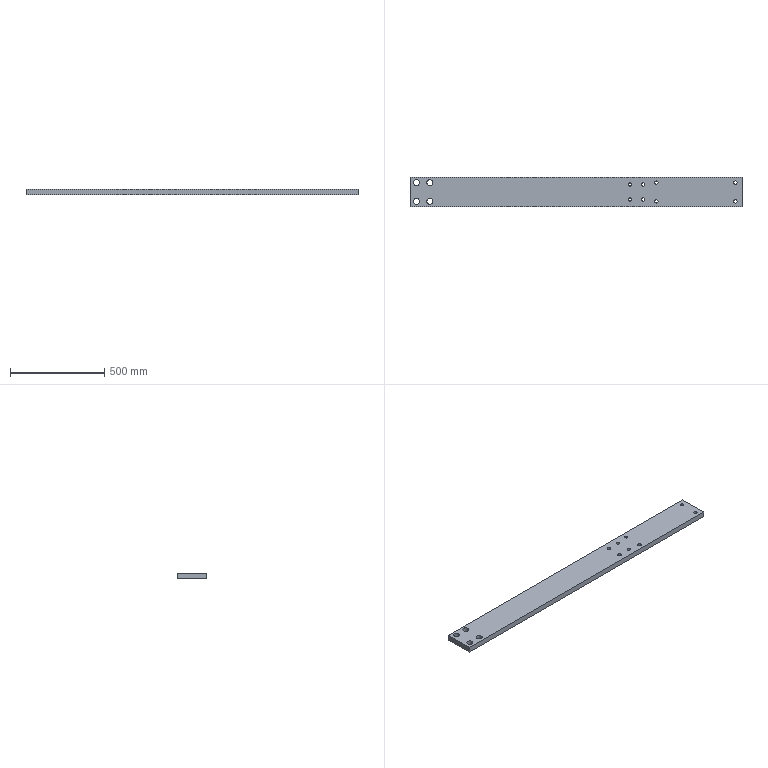Part | NX | features BREP 1 | 1 solid | 30 faces | box 1764 x 158 x 30 mm | volume 8203778 mm3 | cylinder 24 | plane 6 | commonest cylinder face diameters 18 x16 32 x8
STEP:
#1=CARTESIAN_POINT('',(-1230.5,-50.,-15.));
#2=VERTEX_POINT('',#1);
#3=CARTESIAN_POINT('',(-1198.5,-50.,-15.));
#4=VERTEX_POINT('',#3);
#5=CARTESIAN_POINT('',(-1214.5,-50.,-15.));
#6=DIRECTION('',(0.,0.,1.));
#7=DIRECTION('',(-1.,0.,0.));
#8=AXIS2_PLACEMENT_3D('',#5,#6,#7);
#9=CIRCLE('',#8,16.);
#10=EDGE_CURVE('',#2,#4,#9,.T.);
#11=ORIENTED_EDGE('',*,*,#10,.F.);
#12=CARTESIAN_POINT('',(-1230.5,-50.,15.));
#13=VERTEX_POINT('',#12);
#14=CARTESIAN_POINT('',(-1230.5,-50.,-15.));
#15=DIRECTION('',(0.,0.,1.));
#16=VECTOR('',#15,1000.);
#17=LINE('',#14,#16);
#18=EDGE_CURVE('',#2,#13,#17,.T.);
#19=ORIENTED_EDGE('',*,*,#18,.T.);
#20=CARTESIAN_POINT('',(-1198.5,-50.,15.));
#21=VERTEX_POINT('',#20);
#22=CARTESIAN_POINT('',(-1214.5,-50.,15.));
#23=DIRECTION('',(0.,0.,1.));
#24=DIRECTION('',(-1.,0.,0.));
#25=AXIS2_PLACEMENT_3D('',#22,#23,#24);
#26=CIRCLE('',#25,16.);
#27=EDGE_CURVE('',#13,#21,#26,.T.);
#28=ORIENTED_EDGE('',*,*,#27,.T.);
#29=CARTESIAN_POINT('',(-1198.5,-50.,-15.));
#30=DIRECTION('',(0.,0.,1.));
#31=VECTOR('',#30,1000.);
#32=LINE('',#29,#31);
#33=EDGE_CURVE('',#4,#21,#32,.T.);
#34=ORIENTED_EDGE('',*,*,#33,.F.);
#35=EDGE_LOOP('',(#11,#19,#28,#34));
#36=FACE_BOUND('',#35,.T.);
#37=CARTESIAN_POINT('',(-1214.5,-50.,-15.));
#38=DIRECTION('',(0.,0.,1.));
#39=DIRECTION('',(-1.,0.,0.));
#40=AXIS2_PLACEMENT_3D('',#37,#38,#39);
#41=CYLINDRICAL_SURFACE('',#40,16.);
#42=ADVANCED_FACE('',(#36),#41,.F.);
#43=CARTESIAN_POINT('',(-1160.5,-50.,-15.));
#44=VERTEX_POINT('',#43);
#45=CARTESIAN_POINT('',(-1128.5,-50.,-15.));
#46=VERTEX_POINT('',#45);
#47=CARTESIAN_POINT('',(-1144.5,-50.,-15.));
#48=DIRECTION('',(0.,0.,1.));
#49=DIRECTION('',(-1.,0.,0.));
#50=AXIS2_PLACEMENT_3D('',#47,#48,#49);
#51=CIRCLE('',#50,16.);
#52=EDGE_CURVE('',#44,#46,#51,.T.);
#53=ORIENTED_EDGE('',*,*,#52,.F.);
#54=CARTESIAN_POINT('',(-1160.5,-50.,15.));
#55=VERTEX_POINT('',#54);
#56=CARTESIAN_POINT('',(-1160.5,-50.,-15.));
#57=DIRECTION('',(0.,0.,1.));
#58=VECTOR('',#57,1000.);
#59=LINE('',#56,#58);
#60=EDGE_CURVE('',#44,#55,#59,.T.);
#61=ORIENTED_EDGE('',*,*,#60,.T.);
#62=CARTESIAN_POINT('',(-1128.5,-50.,15.));
#63=VERTEX_POINT('',#62);
#64=CARTESIAN_POINT('',(-1144.5,-50.,15.));
#65=DIRECTION('',(0.,0.,1.));
#66=DIRECTION('',(-1.,0.,0.));
#67=AXIS2_PLACEMENT_3D('',#64,#65,#66);
#68=CIRCLE('',#67,16.);
#69=EDGE_CURVE('',#55,#63,#68,.T.);
#70=ORIENTED_EDGE('',*,*,#69,.T.);
#71=CARTESIAN_POINT('',(-1128.5,-50.,-15.));
#72=DIRECTION('',(0.,0.,1.));
#73=VECTOR('',#72,1000.);
#74=LINE('',#71,#73);
#75=EDGE_CURVE('',#46,#63,#74,.T.);
#76=ORIENTED_EDGE('',*,*,#75,.F.);
#77=EDGE_LOOP('',(#53,#61,#70,#76));
#78=FACE_BOUND('',#77,.T.);
#79=CARTESIAN_POINT('',(-1144.5,-50.,-15.));
#80=DIRECTION('',(0.,0.,1.));
#81=DIRECTION('',(-1.,0.,0.));
#82=AXIS2_PLACEMENT_3D('',#79,#80,#81);
#83=CYLINDRICAL_SURFACE('',#82,16.);
#84=ADVANCED_FACE('',(#78),#83,.F.);
#85=CARTESIAN_POINT('',(-1160.5,50.,-15.));
#86=VERTEX_POINT('',#85);
#87=CARTESIAN_POINT('',(-1128.5,50.,-15.));
#88=VERTEX_POINT('',#87);
#89=CARTESIAN_POINT('',(-1144.5,50.,-15.));
#90=DIRECTION('',(0.,0.,1.));
#91=DIRECTION('',(1.,0.,0.));
#92=AXIS2_PLACEMENT_3D('',#89,#90,#91);
#93=CIRCLE('',#92,16.);
#94=EDGE_CURVE('',#86,#88,#93,.T.);
#95=ORIENTED_EDGE('',*,*,#94,.F.);
#96=CARTESIAN_POINT('',(-1160.5,50.,15.));
#97=VERTEX_POINT('',#96);
#98=CARTESIAN_POINT('',(-1160.5,50.,-15.));
#99=DIRECTION('',(0.,0.,1.));
#100=VECTOR('',#99,1000.);
#101=LINE('',#98,#100);
#102=EDGE_CURVE('',#86,#97,#101,.T.);
#103=ORIENTED_EDGE('',*,*,#102,.T.);
#104=CARTESIAN_POINT('',(-1128.5,50.,15.));
#105=VERTEX_POINT('',#104);
#106=CARTESIAN_POINT('',(-1144.5,50.,15.));
#107=DIRECTION('',(0.,0.,1.));
#108=DIRECTION('',(1.,0.,0.));
#109=AXIS2_PLACEMENT_3D('',#106,#107,#108);
#110=CIRCLE('',#109,16.);
#111=EDGE_CURVE('',#97,#105,#110,.T.);
#112=ORIENTED_EDGE('',*,*,#111,.T.);
#113=CARTESIAN_POINT('',(-1128.5,50.,-15.));
#114=DIRECTION('',(0.,0.,1.));
#115=VECTOR('',#114,1000.);
#116=LINE('',#113,#115);
#117=EDGE_CURVE('',#88,#105,#116,.T.);
#118=ORIENTED_EDGE('',*,*,#117,.F.);
#119=EDGE_LOOP('',(#95,#103,#112,#118));
#120=FACE_BOUND('',#119,.T.);
#121=CARTESIAN_POINT('',(-1144.5,50.,-15.));
#122=DIRECTION('',(0.,0.,1.));
#123=DIRECTION('',(-1.,0.,0.));
#124=AXIS2_PLACEMENT_3D('',#121,#122,#123);
#125=CYLINDRICAL_SURFACE('',#124,16.);
#126=ADVANCED_FACE('',(#120),#125,.F.);
#127=CARTESIAN_POINT('',(-1230.5,50.,-15.));
#128=VERTEX_POINT('',#127);
#129=CARTESIAN_POINT('',(-1198.5,50.,-15.));
#130=VERTEX_POINT('',#129);
#131=CARTESIAN_POINT('',(-1214.5,50.,-15.));
#132=DIRECTION('',(0.,0.,1.));
#133=DIRECTION('',(1.,0.,0.));
#134=AXIS2_PLACEMENT_3D('',#131,#132,#133);
#135=CIRCLE('',#134,16.);
#136=EDGE_CURVE('',#128,#130,#135,.T.);
#137=ORIENTED_EDGE('',*,*,#136,.F.);
#138=CARTESIAN_POINT('',(-1230.5,50.,15.));
#139=VERTEX_POINT('',#138);
#140=CARTESIAN_POINT('',(-1230.5,50.,-15.));
#141=DIRECTION('',(0.,0.,1.));
#142=VECTOR('',#141,1000.);
#143=LINE('',#140,#142);
#144=EDGE_CURVE('',#128,#139,#143,.T.);
#145=ORIENTED_EDGE('',*,*,#144,.T.);
#146=CARTESIAN_POINT('',(-1198.5,50.,15.));
#147=VERTEX_POINT('',#146);
#148=CARTESIAN_POINT('',(-1214.5,50.,15.));
#149=DIRECTION('',(0.,0.,1.));
#150=DIRECTION('',(1.,0.,0.));
#151=AXIS2_PLACEMENT_3D('',#148,#149,#150);
#152=CIRCLE('',#151,16.);
#153=EDGE_CURVE('',#139,#147,#152,.T.);
#154=ORIENTED_EDGE('',*,*,#153,.T.);
#155=CARTESIAN_POINT('',(-1198.5,50.,-15.));
#156=DIRECTION('',(0.,0.,1.));
#157=VECTOR('',#156,1000.);
#158=LINE('',#155,#157);
#159=EDGE_CURVE('',#130,#147,#158,.T.);
#160=ORIENTED_EDGE('',*,*,#159,.F.);
#161=EDGE_LOOP('',(#137,#145,#154,#160));
#162=FACE_BOUND('',#161,.T.);
#163=CARTESIAN_POINT('',(-1214.5,50.,-15.));
#164=DIRECTION('',(0.,0.,1.));
#165=DIRECTION('',(-1.,0.,0.));
#166=AXIS2_PLACEMENT_3D('',#163,#164,#165);
#167=CYLINDRICAL_SURFACE('',#166,16.);
#168=ADVANCED_FACE('',(#162),#167,.F.);
#169=CARTESIAN_POINT('',(-89.5,-40.,-15.));
#170=VERTEX_POINT('',#169);
#171=CARTESIAN_POINT('',(-71.5,-40.,-15.));
#172=VERTEX_POINT('',#171);
#173=CARTESIAN_POINT('',(-80.5,-40.,-15.));
#174=DIRECTION('',(0.,0.,1.));
#175=DIRECTION('',(1.,0.,0.));
#176=AXIS2_PLACEMENT_3D('',#173,#174,#175);
#177=CIRCLE('',#176,9.);
#178=EDGE_CURVE('',#170,#172,#177,.T.);
#179=ORIENTED_EDGE('',*,*,#178,.F.);
#180=CARTESIAN_POINT('',(-89.5,-40.,15.));
#181=VERTEX_POINT('',#180);
#182=CARTESIAN_POINT('',(-89.5,-40.,-15.));
#183=DIRECTION('',(0.,0.,1.));
#184=VECTOR('',#183,1000.);
#185=LINE('',#182,#184);
#186=EDGE_CURVE('',#170,#181,#185,.T.);
#187=ORIENTED_EDGE('',*,*,#186,.T.);
#188=CARTESIAN_POINT('',(-71.5,-40.,15.));
#189=VERTEX_POINT('',#188);
#190=CARTESIAN_POINT('',(-80.5,-40.,15.));
#191=DIRECTION('',(0.,0.,1.));
#192=DIRECTION('',(1.,0.,0.));
#193=AXIS2_PLACEMENT_3D('',#190,#191,#192);
#194=CIRCLE('',#193,9.);
#195=EDGE_CURVE('',#181,#189,#194,.T.);
#196=ORIENTED_EDGE('',*,*,#195,.T.);
#197=CARTESIAN_POINT('',(-71.5,-40.,-15.));
#198=DIRECTION('',(0.,0.,1.));
#199=VECTOR('',#198,1000.);
#200=LINE('',#197,#199);
#201=EDGE_CURVE('',#172,#189,#200,.T.);
#202=ORIENTED_EDGE('',*,*,#201,.F.);
#203=EDGE_LOOP('',(#179,#187,#196,#202));
#204=FACE_BOUND('',#203,.T.);
#205=CARTESIAN_POINT('',(-80.5,-40.,-15.));
#206=DIRECTION('',(0.,0.,1.));
#207=DIRECTION('',(-1.,0.,0.));
#208=AXIS2_PLACEMENT_3D('',#205,#206,#207);
#209=CYLINDRICAL_SURFACE('',#208,9.);
#210=ADVANCED_FACE('',(#204),#209,.F.);
#211=CARTESIAN_POINT('',(-19.5,-40.,-15.));
#212=VERTEX_POINT('',#211);
#213=CARTESIAN_POINT('',(-1.5,-40.,-15.));
#214=VERTEX_POINT('',#213);
#215=CARTESIAN_POINT('',(-10.5,-40.,-15.));
#216=DIRECTION('',(0.,0.,1.));
#217=DIRECTION('',(1.,0.,0.));
#218=AXIS2_PLACEMENT_3D('',#215,#216,#217);
#219=CIRCLE('',#218,9.);
#220=EDGE_CURVE('',#212,#214,#219,.T.);
#221=ORIENTED_EDGE('',*,*,#220,.F.);
#222=CARTESIAN_POINT('',(-19.5,-40.,15.));
#223=VERTEX_POINT('',#222);
#224=CARTESIAN_POINT('',(-19.5,-40.,-15.));
#225=DIRECTION('',(0.,0.,1.));
#226=VECTOR('',#225,1000.);
#227=LINE('',#224,#226);
#228=EDGE_CURVE('',#212,#223,#227,.T.);
#229=ORIENTED_EDGE('',*,*,#228,.T.);
#230=CARTESIAN_POINT('',(-1.5,-40.,15.));
#231=VERTEX_POINT('',#230);
#232=CARTESIAN_POINT('',(-10.5,-40.,15.));
#233=DIRECTION('',(0.,0.,1.));
#234=DIRECTION('',(1.,0.,0.));
#235=AXIS2_PLACEMENT_3D('',#232,#233,#234);
#236=CIRCLE('',#235,9.);
#237=EDGE_CURVE('',#223,#231,#236,.T.);
#238=ORIENTED_EDGE('',*,*,#237,.T.);
#239=CARTESIAN_POINT('',(-1.5,-40.,-15.));
#240=DIRECTION('',(0.,0.,1.));
#241=VECTOR('',#240,1000.);
#242=LINE('',#239,#241);
#243=EDGE_CURVE('',#214,#231,#242,.T.);
#244=ORIENTED_EDGE('',*,*,#243,.F.);
#245=EDGE_LOOP('',(#221,#229,#238,#244));
#246=FACE_BOUND('',#245,.T.);
#247=CARTESIAN_POINT('',(-10.5,-40.,-15.));
#248=DIRECTION('',(0.,0.,1.));
#249=DIRECTION('',(-1.,0.,0.));
#250=AXIS2_PLACEMENT_3D('',#247,#248,#249);
#251=CYLINDRICAL_SURFACE('',#250,9.);
#252=ADVANCED_FACE('',(#246),#251,.F.);
#253=CARTESIAN_POINT('',(-89.5,40.,-15.));
#254=VERTEX_POINT('',#253);
#255=CARTESIAN_POINT('',(-71.5,40.,-15.));
#256=VERTEX_POINT('',#255);
#257=CARTESIAN_POINT('',(-80.5,40.,-15.));
#258=DIRECTION('',(0.,0.,1.));
#259=DIRECTION('',(1.,0.,0.));
#260=AXIS2_PLACEMENT_3D('',#257,#258,#259);
#261=CIRCLE('',#260,9.);
#262=EDGE_CURVE('',#254,#256,#261,.T.);
#263=ORIENTED_EDGE('',*,*,#262,.F.);
#264=CARTESIAN_POINT('',(-89.5,40.,15.));
#265=VERTEX_POINT('',#264);
#266=CARTESIAN_POINT('',(-89.5,40.,-15.));
#267=DIRECTION('',(0.,0.,1.));
#268=VECTOR('',#267,1000.);
#269=LINE('',#266,#268);
#270=EDGE_CURVE('',#254,#265,#269,.T.);
#271=ORIENTED_EDGE('',*,*,#270,.T.);
#272=CARTESIAN_POINT('',(-71.5,40.,15.));
#273=VERTEX_POINT('',#272);
#274=CARTESIAN_POINT('',(-80.5,40.,15.));
#275=DIRECTION('',(0.,0.,1.));
#276=DIRECTION('',(1.,0.,0.));
#277=AXIS2_PLACEMENT_3D('',#274,#275,#276);
#278=CIRCLE('',#277,9.);
#279=EDGE_CURVE('',#265,#273,#278,.T.);
#280=ORIENTED_EDGE('',*,*,#279,.T.);
#281=CARTESIAN_POINT('',(-71.5,40.,-15.));
#282=DIRECTION('',(0.,0.,1.));
#283=VECTOR('',#282,1000.);
#284=LINE('',#281,#283);
#285=EDGE_CURVE('',#256,#273,#284,.T.);
#286=ORIENTED_EDGE('',*,*,#285,.F.);
#287=EDGE_LOOP('',(#263,#271,#280,#286));
#288=FACE_BOUND('',#287,.T.);
#289=CARTESIAN_POINT('',(-80.5,40.,-15.));
#290=DIRECTION('',(0.,0.,1.));
#291=DIRECTION('',(-1.,0.,0.));
#292=AXIS2_PLACEMENT_3D('',#289,#290,#291);
#293=CYLINDRICAL_SURFACE('',#292,9.);
#294=ADVANCED_FACE('',(#288),#293,.F.);
#295=CARTESIAN_POINT('',(-19.5,40.,-15.));
#296=VERTEX_POINT('',#295);
#297=CARTESIAN_POINT('',(-1.5,40.,-15.));
#298=VERTEX_POINT('',#297);
#299=CARTESIAN_POINT('',(-10.5,40.,-15.));
#300=DIRECTION('',(0.,0.,1.));
#301=DIRECTION('',(1.,0.,0.));
#302=AXIS2_PLACEMENT_3D('',#299,#300,#301);
#303=CIRCLE('',#302,9.);
#304=EDGE_CURVE('',#296,#298,#303,.T.);
#305=ORIENTED_EDGE('',*,*,#304,.F.);
#306=CARTESIAN_POINT('',(-19.5,40.,15.));
#307=VERTEX_POINT('',#306);
#308=CARTESIAN_POINT('',(-19.5,40.,-15.));
#309=DIRECTION('',(0.,0.,1.));
#310=VECTOR('',#309,1000.);
#311=LINE('',#308,#310);
#312=EDGE_CURVE('',#296,#307,#311,.T.);
#313=ORIENTED_EDGE('',*,*,#312,.T.);
#314=CARTESIAN_POINT('',(-1.5,40.,15.));
#315=VERTEX_POINT('',#314);
#316=CARTESIAN_POINT('',(-10.5,40.,15.));
#317=DIRECTION('',(0.,0.,1.));
#318=DIRECTION('',(1.,0.,0.));
#319=AXIS2_PLACEMENT_3D('',#316,#317,#318);
#320=CIRCLE('',#319,9.);
#321=EDGE_CURVE('',#307,#315,#320,.T.);
#322=ORIENTED_EDGE('',*,*,#321,.T.);
#323=CARTESIAN_POINT('',(-1.5,40.,-15.));
#324=DIRECTION('',(0.,0.,1.));
#325=VECTOR('',#324,1000.);
#326=LINE('',#323,#325);
#327=EDGE_CURVE('',#298,#315,#326,.T.);
#328=ORIENTED_EDGE('',*,*,#327,.F.);
#329=EDGE_LOOP('',(#305,#313,#322,#328));
#330=FACE_BOUND('',#329,.T.);
#331=CARTESIAN_POINT('',(-10.5,40.,-15.));
#332=DIRECTION('',(0.,0.,1.));
#333=DIRECTION('',(-1.,0.,0.));
#334=AXIS2_PLACEMENT_3D('',#331,#332,#333);
#335=CYLINDRICAL_SURFACE('',#334,9.);
#336=ADVANCED_FACE('',(#330),#335,.F.);
#337=CARTESIAN_POINT('',(50.5,-50.,-15.));
#338=VERTEX_POINT('',#337);
#339=CARTESIAN_POINT('',(68.5,-50.,-15.));
#340=VERTEX_POINT('',#339);
#341=CARTESIAN_POINT('',(59.5,-50.,-15.));
#342=DIRECTION('',(0.,0.,1.));
#343=DIRECTION('',(1.,0.,0.));
#344=AXIS2_PLACEMENT_3D('',#341,#342,#343);
#345=CIRCLE('',#344,9.);
#346=EDGE_CURVE('',#338,#340,#345,.T.);
#347=ORIENTED_EDGE('',*,*,#346,.F.);
#348=CARTESIAN_POINT('',(50.5,-50.,15.));
#349=VERTEX_POINT('',#348);
#350=CARTESIAN_POINT('',(50.5,-50.,-15.));
#351=DIRECTION('',(0.,0.,1.));
#352=VECTOR('',#351,1000.);
#353=LINE('',#350,#352);
#354=EDGE_CURVE('',#338,#349,#353,.T.);
#355=ORIENTED_EDGE('',*,*,#354,.T.);
#356=CARTESIAN_POINT('',(68.5,-50.,15.));
#357=VERTEX_POINT('',#356);
#358=CARTESIAN_POINT('',(59.5,-50.,15.));
#359=DIRECTION('',(0.,0.,1.));
#360=DIRECTION('',(1.,0.,0.));
#361=AXIS2_PLACEMENT_3D('',#358,#359,#360);
#362=CIRCLE('',#361,9.);
#363=EDGE_CURVE('',#349,#357,#362,.T.);
#364=ORIENTED_EDGE('',*,*,#363,.T.);
#365=CARTESIAN_POINT('',(68.5,-50.,-15.));
#366=DIRECTION('',(0.,0.,1.));
#367=VECTOR('',#366,1000.);
#368=LINE('',#365,#367);
#369=EDGE_CURVE('',#340,#357,#368,.T.);
#370=ORIENTED_EDGE('',*,*,#369,.F.);
#371=EDGE_LOOP('',(#347,#355,#364,#370));
#372=FACE_BOUND('',#371,.T.);
#373=CARTESIAN_POINT('',(59.5,-50.,-15.));
#374=DIRECTION('',(0.,0.,1.));
#375=DIRECTION('',(-1.,0.,0.));
#376=AXIS2_PLACEMENT_3D('',#373,#374,#375);
#377=CYLINDRICAL_SURFACE('',#376,9.);
#378=ADVANCED_FACE('',(#372),#377,.F.);
#379=CARTESIAN_POINT('',(50.5,50.,-15.));
#380=VERTEX_POINT('',#379);
#381=CARTESIAN_POINT('',(68.5,50.,-15.));
#382=VERTEX_POINT('',#381);
#383=CARTESIAN_POINT('',(59.5,50.,-15.));
#384=DIRECTION('',(0.,0.,1.));
#385=DIRECTION('',(-1.,0.,0.));
#386=AXIS2_PLACEMENT_3D('',#383,#384,#385);
#387=CIRCLE('',#386,9.);
#388=EDGE_CURVE('',#380,#382,#387,.T.);
#389=ORIENTED_EDGE('',*,*,#388,.F.);
#390=CARTESIAN_POINT('',(50.5,50.,15.));
#391=VERTEX_POINT('',#390);
#392=CARTESIAN_POINT('',(50.5,50.,-15.));
#393=DIRECTION('',(0.,0.,1.));
#394=VECTOR('',#393,1000.);
#395=LINE('',#392,#394);
#396=EDGE_CURVE('',#380,#391,#395,.T.);
#397=ORIENTED_EDGE('',*,*,#396,.T.);
#398=CARTESIAN_POINT('',(68.5,50.,15.));
#399=VERTEX_POINT('',#398);
#400=CARTESIAN_POINT('',(59.5,50.,15.));
#401=DIRECTION('',(0.,0.,1.));
#402=DIRECTION('',(-1.,0.,0.));
#403=AXIS2_PLACEMENT_3D('',#400,#401,#402);
#404=CIRCLE('',#403,9.);
#405=EDGE_CURVE('',#391,#399,#404,.T.);
#406=ORIENTED_EDGE('',*,*,#405,.T.);
#407=CARTESIAN_POINT('',(68.5,50.,-15.));
#408=DIRECTION('',(0.,0.,1.));
#409=VECTOR('',#408,1000.);
#410=LINE('',#407,#409);
#411=EDGE_CURVE('',#382,#399,#410,.T.);
#412=ORIENTED_EDGE('',*,*,#411,.F.);
#413=EDGE_LOOP('',(#389,#397,#406,#412));
#414=FACE_BOUND('',#413,.T.);
#415=CARTESIAN_POINT('',(59.5,50.,-15.));
#416=DIRECTION('',(0.,0.,1.));
#417=DIRECTION('',(-1.,0.,0.));
#418=AXIS2_PLACEMENT_3D('',#415,#416,#417);
#419=CYLINDRICAL_SURFACE('',#418,9.);
#420=ADVANCED_FACE('',(#414),#419,.F.);
#421=CARTESIAN_POINT('',(470.5,-50.,-15.));
#422=VERTEX_POINT('',#421);
#423=CARTESIAN_POINT('',(488.5,-50.,-15.));
#424=VERTEX_POINT('',#423);
#425=CARTESIAN_POINT('',(479.5,-50.,-15.));
#426=DIRECTION('',(0.,0.,1.));
#427=DIRECTION('',(-1.,0.,0.));
#428=AXIS2_PLACEMENT_3D('',#425,#426,#427);
#429=CIRCLE('',#428,9.);
#430=EDGE_CURVE('',#422,#424,#429,.T.);
#431=ORIENTED_EDGE('',*,*,#430,.F.);
#432=CARTESIAN_POINT('',(470.5,-50.,15.));
#433=VERTEX_POINT('',#432);
#434=CARTESIAN_POINT('',(470.5,-50.,-15.));
#435=DIRECTION('',(0.,0.,1.));
#436=VECTOR('',#435,1000.);
#437=LINE('',#434,#436);
#438=EDGE_CURVE('',#422,#433,#437,.T.);
#439=ORIENTED_EDGE('',*,*,#438,.T.);
#440=CARTESIAN_POINT('',(488.5,-50.,15.));
#441=VERTEX_POINT('',#440);
#442=CARTESIAN_POINT('',(479.5,-50.,15.));
#443=DIRECTION('',(0.,0.,1.));
#444=DIRECTION('',(-1.,0.,0.));
#445=AXIS2_PLACEMENT_3D('',#442,#443,#444);
#446=CIRCLE('',#445,9.);
#447=EDGE_CURVE('',#433,#441,#446,.T.);
#448=ORIENTED_EDGE('',*,*,#447,.T.);
#449=CARTESIAN_POINT('',(488.5,-50.,-15.));
#450=DIRECTION('',(0.,0.,1.));
#451=VECTOR('',#450,1000.);
#452=LINE('',#449,#451);
#453=EDGE_CURVE('',#424,#441,#452,.T.);
#454=ORIENTED_EDGE('',*,*,#453,.F.);
#455=EDGE_LOOP('',(#431,#439,#448,#454));
#456=FACE_BOUND('',#455,.T.);
#457=CARTESIAN_POINT('',(479.5,-50.,-15.));
#458=DIRECTION('',(0.,0.,1.));
#459=DIRECTION('',(-1.,0.,0.));
#460=AXIS2_PLACEMENT_3D('',#457,#458,#459);
#461=CYLINDRICAL_SURFACE('',#460,9.);
#462=ADVANCED_FACE('',(#456),#461,.F.);
#463=CARTESIAN_POINT('',(470.5,50.,-15.));
#464=VERTEX_POINT('',#463);
#465=CARTESIAN_POINT('',(488.5,50.,-15.));
#466=VERTEX_POINT('',#465);
#467=CARTESIAN_POINT('',(479.5,50.,-15.));
#468=DIRECTION('',(0.,0.,1.));
#469=DIRECTION('',(1.,0.,0.));
#470=AXIS2_PLACEMENT_3D('',#467,#468,#469);
#471=CIRCLE('',#470,9.);
#472=EDGE_CURVE('',#464,#466,#471,.T.);
#473=ORIENTED_EDGE('',*,*,#472,.F.);
#474=CARTESIAN_POINT('',(470.5,50.,15.));
#475=VERTEX_POINT('',#474);
#476=CARTESIAN_POINT('',(470.5,50.,-15.));
#477=DIRECTION('',(0.,0.,1.));
#478=VECTOR('',#477,1000.);
#479=LINE('',#476,#478);
#480=EDGE_CURVE('',#464,#475,#479,.T.);
#481=ORIENTED_EDGE('',*,*,#480,.T.);
#482=CARTESIAN_POINT('',(488.5,50.,15.));
#483=VERTEX_POINT('',#482);
#484=CARTESIAN_POINT('',(479.5,50.,15.));
#485=DIRECTION('',(0.,0.,1.));
#486=DIRECTION('',(1.,0.,0.));
#487=AXIS2_PLACEMENT_3D('',#484,#485,#486);
#488=CIRCLE('',#487,9.);
#489=EDGE_CURVE('',#475,#483,#488,.T.);
#490=ORIENTED_EDGE('',*,*,#489,.T.);
#491=CARTESIAN_POINT('',(488.5,50.,-15.));
#492=DIRECTION('',(0.,0.,1.));
#493=VECTOR('',#492,1000.);
#494=LINE('',#491,#493);
#495=EDGE_CURVE('',#466,#483,#494,.T.);
#496=ORIENTED_EDGE('',*,*,#495,.F.);
#497=EDGE_LOOP('',(#473,#481,#490,#496));
#498=FACE_BOUND('',#497,.T.);
#499=CARTESIAN_POINT('',(479.5,50.,-15.));
#500=DIRECTION('',(0.,0.,1.));
#501=DIRECTION('',(-1.,0.,0.));
#502=AXIS2_PLACEMENT_3D('',#499,#500,#501);
#503=CYLINDRICAL_SURFACE('',#502,9.);
#504=ADVANCED_FACE('',(#498),#503,.F.);
#505=CARTESIAN_POINT('',(-1249.5,79.,-15.));
#506=VERTEX_POINT('',#505);
#507=CARTESIAN_POINT('',(-1249.5,-79.,-15.));
#508=VERTEX_POINT('',#507);
#509=CARTESIAN_POINT('',(-1249.5,79.,-15.));
#510=DIRECTION('',(0.,-1.,0.));
#511=VECTOR('',#510,1000.);
#512=LINE('',#509,#511);
#513=EDGE_CURVE('',#506,#508,#512,.T.);
#514=ORIENTED_EDGE('',*,*,#513,.T.);
#515=CARTESIAN_POINT('',(-1249.5,-79.,15.));
#516=VERTEX_POINT('',#515);
#517=CARTESIAN_POINT('',(-1249.5,-79.,15.));
#518=DIRECTION('',(0.,0.,-1.));
#519=VECTOR('',#518,1000.);
#520=LINE('',#517,#519);
#521=EDGE_CURVE('',#516,#508,#520,.T.);
#522=ORIENTED_EDGE('',*,*,#521,.F.);
#523=CARTESIAN_POINT('',(-1249.5,79.,15.));
#524=VERTEX_POINT('',#523);
#525=CARTESIAN_POINT('',(-1249.5,79.,15.));
#526=DIRECTION('',(0.,-1.,0.));
#527=VECTOR('',#526,1000.);
#528=LINE('',#525,#527);
#529=EDGE_CURVE('',#524,#516,#528,.T.);
#530=ORIENTED_EDGE('',*,*,#529,.F.);
#531=CARTESIAN_POINT('',(-1249.5,79.,15.));
#532=DIRECTION('',(0.,0.,-1.));
#533=VECTOR('',#532,1000.);
#534=LINE('',#531,#533);
#535=EDGE_CURVE('',#524,#506,#534,.T.);
#536=ORIENTED_EDGE('',*,*,#535,.T.);
#537=EDGE_LOOP('',(#514,#522,#530,#536));
#538=FACE_BOUND('',#537,.T.);
#539=CARTESIAN_POINT('',(-1249.5,79.,15.));
#540=DIRECTION('',(1.,0.,0.));
#541=DIRECTION('',(0.,0.,1.));
#542=AXIS2_PLACEMENT_3D('',#539,#540,#541);
#543=PLANE('',#542);
#544=ADVANCED_FACE('',(#538),#543,.F.);
#545=CARTESIAN_POINT('',(514.5,-79.,-15.));
#546=VERTEX_POINT('',#545);
#547=CARTESIAN_POINT('',(-1249.5,-79.,-15.));
#548=DIRECTION('',(1.,0.,0.));
#549=VECTOR('',#548,1000.);
#550=LINE('',#547,#549);
#551=EDGE_CURVE('',#508,#546,#550,.T.);
#552=ORIENTED_EDGE('',*,*,#551,.T.);
#553=CARTESIAN_POINT('',(514.5,-79.,15.));
#554=VERTEX_POINT('',#553);
#555=CARTESIAN_POINT('',(514.5,-79.,-15.));
#556=DIRECTION('',(0.,0.,1.));
#557=VECTOR('',#556,1000.);
#558=LINE('',#555,#557);
#559=EDGE_CURVE('',#546,#554,#558,.T.);
#560=ORIENTED_EDGE('',*,*,#559,.T.);
#561=CARTESIAN_POINT('',(-1249.5,-79.,15.));
#562=DIRECTION('',(1.,0.,0.));
#563=VECTOR('',#562,1000.);
#564=LINE('',#561,#563);
#565=EDGE_CURVE('',#516,#554,#564,.T.);
#566=ORIENTED_EDGE('',*,*,#565,.F.);
#567=ORIENTED_EDGE('',*,*,#521,.T.);
#568=EDGE_LOOP('',(#552,#560,#566,#567));
#569=FACE_BOUND('',#568,.T.);
#570=CARTESIAN_POINT('',(-1249.5,-79.,15.));
#571=DIRECTION('',(0.,1.,0.));
#572=DIRECTION('',(0.,0.,-1.));
#573=AXIS2_PLACEMENT_3D('',#570,#571,#572);
#574=PLANE('',#573);
#575=ADVANCED_FACE('',(#569),#574,.F.);
#576=CARTESIAN_POINT('',(514.5,79.,15.));
#577=VERTEX_POINT('',#576);
#578=CARTESIAN_POINT('',(-1249.5,79.,15.));
#579=DIRECTION('',(-1.,0.,0.));
#580=VECTOR('',#579,1000.);
#581=LINE('',#578,#580);
#582=EDGE_CURVE('',#577,#524,#581,.T.);
#583=ORIENTED_EDGE('',*,*,#582,.F.);
#584=CARTESIAN_POINT('',(514.5,79.,-15.));
#585=VERTEX_POINT('',#584);
#586=CARTESIAN_POINT('',(514.5,79.,-15.));
#587=DIRECTION('',(0.,0.,1.));
#588=VECTOR('',#587,1000.);
#589=LINE('',#586,#588);
#590=EDGE_CURVE('',#585,#577,#589,.T.);
#591=ORIENTED_EDGE('',*,*,#590,.F.);
#592=CARTESIAN_POINT('',(-1249.5,79.,-15.));
#593=DIRECTION('',(-1.,0.,0.));
#594=VECTOR('',#593,1000.);
#595=LINE('',#592,#594);
#596=EDGE_CURVE('',#585,#506,#595,.T.);
#597=ORIENTED_EDGE('',*,*,#596,.T.);
#598=ORIENTED_EDGE('',*,*,#535,.F.);
#599=EDGE_LOOP('',(#583,#591,#597,#598));
#600=FACE_BOUND('',#599,.T.);
#601=CARTESIAN_POINT('',(-1249.5,79.,15.));
#602=DIRECTION('',(0.,-1.,0.));
#603=DIRECTION('',(0.,0.,1.));
#604=AXIS2_PLACEMENT_3D('',#601,#602,#603);
#605=PLANE('',#604);
#606=ADVANCED_FACE('',(#600),#605,.F.);
#607=CARTESIAN_POINT('',(514.5,79.,15.));
#608=DIRECTION('',(0.,-1.,0.));
#609=VECTOR('',#608,1000.);
#610=LINE('',#607,#609);
#611=EDGE_CURVE('',#577,#554,#610,.T.);
#612=ORIENTED_EDGE('',*,*,#611,.F.);
#613=ORIENTED_EDGE('',*,*,#582,.T.);
#614=ORIENTED_EDGE('',*,*,#529,.T.);
#615=ORIENTED_EDGE('',*,*,#565,.T.);
#616=EDGE_LOOP('',(#612,#613,#614,#615));
#617=FACE_BOUND('',#616,.T.);
#618=CARTESIAN_POINT('',(-1214.5,-50.,15.));
#619=DIRECTION('',(0.,0.,1.));
#620=DIRECTION('',(-1.,0.,0.));
#621=AXIS2_PLACEMENT_3D('',#618,#619,#620);
#622=CIRCLE('',#621,16.);
#623=EDGE_CURVE('',#21,#13,#622,.T.);
#624=ORIENTED_EDGE('',*,*,#623,.F.);
#625=ORIENTED_EDGE('',*,*,#27,.F.);
#626=EDGE_LOOP('',(#624,#625));
#627=FACE_BOUND('',#626,.T.);
#628=CARTESIAN_POINT('',(-1144.5,-50.,15.));
#629=DIRECTION('',(0.,0.,1.));
#630=DIRECTION('',(-1.,0.,0.));
#631=AXIS2_PLACEMENT_3D('',#628,#629,#630);
#632=CIRCLE('',#631,16.);
#633=EDGE_CURVE('',#63,#55,#632,.T.);
#634=ORIENTED_EDGE('',*,*,#633,.F.);
#635=ORIENTED_EDGE('',*,*,#69,.F.);
#636=EDGE_LOOP('',(#634,#635));
#637=FACE_BOUND('',#636,.T.);
#638=CARTESIAN_POINT('',(-1144.5,50.,15.));
#639=DIRECTION('',(0.,0.,1.));
#640=DIRECTION('',(1.,0.,0.));
#641=AXIS2_PLACEMENT_3D('',#638,#639,#640);
#642=CIRCLE('',#641,16.);
#643=EDGE_CURVE('',#105,#97,#642,.T.);
#644=ORIENTED_EDGE('',*,*,#643,.F.);
#645=ORIENTED_EDGE('',*,*,#111,.F.);
#646=EDGE_LOOP('',(#644,#645));
#647=FACE_BOUND('',#646,.T.);
#648=CARTESIAN_POINT('',(-1214.5,50.,15.));
#649=DIRECTION('',(0.,0.,1.));
#650=DIRECTION('',(1.,0.,0.));
#651=AXIS2_PLACEMENT_3D('',#648,#649,#650);
#652=CIRCLE('',#651,16.);
#653=EDGE_CURVE('',#147,#139,#652,.T.);
#654=ORIENTED_EDGE('',*,*,#653,.F.);
#655=ORIENTED_EDGE('',*,*,#153,.F.);
#656=EDGE_LOOP('',(#654,#655));
#657=FACE_BOUND('',#656,.T.);
#658=CARTESIAN_POINT('',(-80.5,-40.,15.));
#659=DIRECTION('',(0.,0.,1.));
#660=DIRECTION('',(1.,0.,0.));
#661=AXIS2_PLACEMENT_3D('',#658,#659,#660);
#662=CIRCLE('',#661,9.);
#663=EDGE_CURVE('',#189,#181,#662,.T.);
#664=ORIENTED_EDGE('',*,*,#663,.F.);
#665=ORIENTED_EDGE('',*,*,#195,.F.);
#666=EDGE_LOOP('',(#664,#665));
#667=FACE_BOUND('',#666,.T.);
#668=CARTESIAN_POINT('',(-10.5,-40.,15.));
#669=DIRECTION('',(0.,0.,1.));
#670=DIRECTION('',(1.,0.,0.));
#671=AXIS2_PLACEMENT_3D('',#668,#669,#670);
#672=CIRCLE('',#671,9.);
#673=EDGE_CURVE('',#231,#223,#672,.T.);
#674=ORIENTED_EDGE('',*,*,#673,.F.);
#675=ORIENTED_EDGE('',*,*,#237,.F.);
#676=EDGE_LOOP('',(#674,#675));
#677=FACE_BOUND('',#676,.T.);
#678=CARTESIAN_POINT('',(-80.5,40.,15.));
#679=DIRECTION('',(0.,0.,1.));
#680=DIRECTION('',(1.,0.,0.));
#681=AXIS2_PLACEMENT_3D('',#678,#679,#680);
#682=CIRCLE('',#681,9.);
#683=EDGE_CURVE('',#273,#265,#682,.T.);
#684=ORIENTED_EDGE('',*,*,#683,.F.);
#685=ORIENTED_EDGE('',*,*,#279,.F.);
#686=EDGE_LOOP('',(#684,#685));
#687=FACE_BOUND('',#686,.T.);
#688=CARTESIAN_POINT('',(-10.5,40.,15.));
#689=DIRECTION('',(0.,0.,1.));
#690=DIRECTION('',(1.,0.,0.));
#691=AXIS2_PLACEMENT_3D('',#688,#689,#690);
#692=CIRCLE('',#691,9.);
#693=EDGE_CURVE('',#315,#307,#692,.T.);
#694=ORIENTED_EDGE('',*,*,#693,.F.);
#695=ORIENTED_EDGE('',*,*,#321,.F.);
#696=EDGE_LOOP('',(#694,#695));
#697=FACE_BOUND('',#696,.T.);
#698=CARTESIAN_POINT('',(59.5,-50.,15.));
#699=DIRECTION('',(0.,0.,1.));
#700=DIRECTION('',(1.,0.,0.));
#701=AXIS2_PLACEMENT_3D('',#698,#699,#700);
#702=CIRCLE('',#701,9.);
#703=EDGE_CURVE('',#357,#349,#702,.T.);
#704=ORIENTED_EDGE('',*,*,#703,.F.);
#705=ORIENTED_EDGE('',*,*,#363,.F.);
#706=EDGE_LOOP('',(#704,#705));
#707=FACE_BOUND('',#706,.T.);
#708=CARTESIAN_POINT('',(59.5,50.,15.));
#709=DIRECTION('',(0.,0.,1.));
#710=DIRECTION('',(-1.,0.,0.));
#711=AXIS2_PLACEMENT_3D('',#708,#709,#710);
#712=CIRCLE('',#711,9.);
#713=EDGE_CURVE('',#399,#391,#712,.T.);
#714=ORIENTED_EDGE('',*,*,#713,.F.);
#715=ORIENTED_EDGE('',*,*,#405,.F.);
#716=EDGE_LOOP('',(#714,#715));
#717=FACE_BOUND('',#716,.T.);
#718=CARTESIAN_POINT('',(479.5,-50.,15.));
#719=DIRECTION('',(0.,0.,1.));
#720=DIRECTION('',(-1.,0.,0.));
#721=AXIS2_PLACEMENT_3D('',#718,#719,#720);
#722=CIRCLE('',#721,9.);
#723=EDGE_CURVE('',#441,#433,#722,.T.);
#724=ORIENTED_EDGE('',*,*,#723,.F.);
#725=ORIENTED_EDGE('',*,*,#447,.F.);
#726=EDGE_LOOP('',(#724,#725));
#727=FACE_BOUND('',#726,.T.);
#728=CARTESIAN_POINT('',(479.5,50.,15.));
#729=DIRECTION('',(0.,0.,1.));
#730=DIRECTION('',(1.,0.,0.));
#731=AXIS2_PLACEMENT_3D('',#728,#729,#730);
#732=CIRCLE('',#731,9.);
#733=EDGE_CURVE('',#483,#475,#732,.T.);
#734=ORIENTED_EDGE('',*,*,#733,.F.);
#735=ORIENTED_EDGE('',*,*,#489,.F.);
#736=EDGE_LOOP('',(#734,#735));
#737=FACE_BOUND('',#736,.T.);
#738=CARTESIAN_POINT('',(-1249.5,-79.,15.));
#739=DIRECTION('',(0.,0.,1.));
#740=DIRECTION('',(-1.,0.,0.));
#741=AXIS2_PLACEMENT_3D('',#738,#739,#740);
#742=PLANE('',#741);
#743=ADVANCED_FACE('',(#617,#627,#637,#647,#657,#667,#677,#687,#697,#707,#717,#727,#737),#742,.T.);
#744=CARTESIAN_POINT('',(-1214.5,-50.,-15.));
#745=DIRECTION('',(0.,0.,1.));
#746=DIRECTION('',(-1.,0.,0.));
#747=AXIS2_PLACEMENT_3D('',#744,#745,#746);
#748=CIRCLE('',#747,16.);
#749=EDGE_CURVE('',#4,#2,#748,.T.);
#750=ORIENTED_EDGE('',*,*,#749,.T.);
#751=ORIENTED_EDGE('',*,*,#10,.T.);
#752=EDGE_LOOP('',(#750,#751));
#753=FACE_BOUND('',#752,.T.);
#754=CARTESIAN_POINT('',(-1144.5,-50.,-15.));
#755=DIRECTION('',(0.,0.,1.));
#756=DIRECTION('',(-1.,0.,0.));
#757=AXIS2_PLACEMENT_3D('',#754,#755,#756);
#758=CIRCLE('',#757,16.);
#759=EDGE_CURVE('',#46,#44,#758,.T.);
#760=ORIENTED_EDGE('',*,*,#759,.T.);
#761=ORIENTED_EDGE('',*,*,#52,.T.);
#762=EDGE_LOOP('',(#760,#761));
#763=FACE_BOUND('',#762,.T.);
#764=CARTESIAN_POINT('',(-1144.5,50.,-15.));
#765=DIRECTION('',(0.,0.,1.));
#766=DIRECTION('',(1.,0.,0.));
#767=AXIS2_PLACEMENT_3D('',#764,#765,#766);
#768=CIRCLE('',#767,16.);
#769=EDGE_CURVE('',#88,#86,#768,.T.);
#770=ORIENTED_EDGE('',*,*,#769,.T.);
#771=ORIENTED_EDGE('',*,*,#94,.T.);
#772=EDGE_LOOP('',(#770,#771));
#773=FACE_BOUND('',#772,.T.);
#774=CARTESIAN_POINT('',(-1214.5,50.,-15.));
#775=DIRECTION('',(0.,0.,1.));
#776=DIRECTION('',(1.,0.,0.));
#777=AXIS2_PLACEMENT_3D('',#774,#775,#776);
#778=CIRCLE('',#777,16.);
#779=EDGE_CURVE('',#130,#128,#778,.T.);
#780=ORIENTED_EDGE('',*,*,#779,.T.);
#781=ORIENTED_EDGE('',*,*,#136,.T.);
#782=EDGE_LOOP('',(#780,#781));
#783=FACE_BOUND('',#782,.T.);
#784=CARTESIAN_POINT('',(-80.5,-40.,-15.));
#785=DIRECTION('',(0.,0.,1.));
#786=DIRECTION('',(1.,0.,0.));
#787=AXIS2_PLACEMENT_3D('',#784,#785,#786);
#788=CIRCLE('',#787,9.);
#789=EDGE_CURVE('',#172,#170,#788,.T.);
#790=ORIENTED_EDGE('',*,*,#789,.T.);
#791=ORIENTED_EDGE('',*,*,#178,.T.);
#792=EDGE_LOOP('',(#790,#791));
#793=FACE_BOUND('',#792,.T.);
#794=CARTESIAN_POINT('',(-10.5,-40.,-15.));
#795=DIRECTION('',(0.,0.,1.));
#796=DIRECTION('',(1.,0.,0.));
#797=AXIS2_PLACEMENT_3D('',#794,#795,#796);
#798=CIRCLE('',#797,9.);
#799=EDGE_CURVE('',#214,#212,#798,.T.);
#800=ORIENTED_EDGE('',*,*,#799,.T.);
#801=ORIENTED_EDGE('',*,*,#220,.T.);
#802=EDGE_LOOP('',(#800,#801));
#803=FACE_BOUND('',#802,.T.);
#804=CARTESIAN_POINT('',(-80.5,40.,-15.));
#805=DIRECTION('',(0.,0.,1.));
#806=DIRECTION('',(1.,0.,0.));
#807=AXIS2_PLACEMENT_3D('',#804,#805,#806);
#808=CIRCLE('',#807,9.);
#809=EDGE_CURVE('',#256,#254,#808,.T.);
#810=ORIENTED_EDGE('',*,*,#809,.T.);
#811=ORIENTED_EDGE('',*,*,#262,.T.);
#812=EDGE_LOOP('',(#810,#811));
#813=FACE_BOUND('',#812,.T.);
#814=CARTESIAN_POINT('',(-10.5,40.,-15.));
#815=DIRECTION('',(0.,0.,1.));
#816=DIRECTION('',(1.,0.,0.));
#817=AXIS2_PLACEMENT_3D('',#814,#815,#816);
#818=CIRCLE('',#817,9.);
#819=EDGE_CURVE('',#298,#296,#818,.T.);
#820=ORIENTED_EDGE('',*,*,#819,.T.);
#821=ORIENTED_EDGE('',*,*,#304,.T.);
#822=EDGE_LOOP('',(#820,#821));
#823=FACE_BOUND('',#822,.T.);
#824=CARTESIAN_POINT('',(59.5,-50.,-15.));
#825=DIRECTION('',(0.,0.,1.));
#826=DIRECTION('',(1.,0.,0.));
#827=AXIS2_PLACEMENT_3D('',#824,#825,#826);
#828=CIRCLE('',#827,9.);
#829=EDGE_CURVE('',#340,#338,#828,.T.);
#830=ORIENTED_EDGE('',*,*,#829,.T.);
#831=ORIENTED_EDGE('',*,*,#346,.T.);
#832=EDGE_LOOP('',(#830,#831));
#833=FACE_BOUND('',#832,.T.);
#834=CARTESIAN_POINT('',(59.5,50.,-15.));
#835=DIRECTION('',(0.,0.,1.));
#836=DIRECTION('',(-1.,0.,0.));
#837=AXIS2_PLACEMENT_3D('',#834,#835,#836);
#838=CIRCLE('',#837,9.);
#839=EDGE_CURVE('',#382,#380,#838,.T.);
#840=ORIENTED_EDGE('',*,*,#839,.T.);
#841=ORIENTED_EDGE('',*,*,#388,.T.);
#842=EDGE_LOOP('',(#840,#841));
#843=FACE_BOUND('',#842,.T.);
#844=CARTESIAN_POINT('',(479.5,-50.,-15.));
#845=DIRECTION('',(0.,0.,1.));
#846=DIRECTION('',(-1.,0.,0.));
#847=AXIS2_PLACEMENT_3D('',#844,#845,#846);
#848=CIRCLE('',#847,9.);
#849=EDGE_CURVE('',#424,#422,#848,.T.);
#850=ORIENTED_EDGE('',*,*,#849,.T.);
#851=ORIENTED_EDGE('',*,*,#430,.T.);
#852=EDGE_LOOP('',(#850,#851));
#853=FACE_BOUND('',#852,.T.);
#854=CARTESIAN_POINT('',(479.5,50.,-15.));
#855=DIRECTION('',(0.,0.,1.));
#856=DIRECTION('',(1.,0.,0.));
#857=AXIS2_PLACEMENT_3D('',#854,#855,#856);
#858=CIRCLE('',#857,9.);
#859=EDGE_CURVE('',#466,#464,#858,.T.);
#860=ORIENTED_EDGE('',*,*,#859,.T.);
#861=ORIENTED_EDGE('',*,*,#472,.T.);
#862=EDGE_LOOP('',(#860,#861));
#863=FACE_BOUND('',#862,.T.);
#864=ORIENTED_EDGE('',*,*,#596,.F.);
#865=CARTESIAN_POINT('',(514.5,79.,-15.));
#866=DIRECTION('',(0.,-1.,0.));
#867=VECTOR('',#866,1000.);
#868=LINE('',#865,#867);
#869=EDGE_CURVE('',#585,#546,#868,.T.);
#870=ORIENTED_EDGE('',*,*,#869,.T.);
#871=ORIENTED_EDGE('',*,*,#551,.F.);
#872=ORIENTED_EDGE('',*,*,#513,.F.);
#873=EDGE_LOOP('',(#864,#870,#871,#872));
#874=FACE_BOUND('',#873,.T.);
#875=CARTESIAN_POINT('',(-1249.5,-79.,-15.));
#876=DIRECTION('',(0.,0.,1.));
#877=DIRECTION('',(-1.,0.,0.));
#878=AXIS2_PLACEMENT_3D('',#875,#876,#877);
#879=PLANE('',#878);
#880=ADVANCED_FACE('',(#753,#763,#773,#783,#793,#803,#813,#823,#833,#843,#853,#863,#874),#879,.F.);
#881=ORIENTED_EDGE('',*,*,#480,.F.);
#882=ORIENTED_EDGE('',*,*,#859,.F.);
#883=ORIENTED_EDGE('',*,*,#495,.T.);
#884=ORIENTED_EDGE('',*,*,#733,.T.);
#885=EDGE_LOOP('',(#881,#882,#883,#884));
#886=FACE_BOUND('',#885,.T.);
#887=CARTESIAN_POINT('',(479.5,50.,-15.));
#888=DIRECTION('',(0.,0.,1.));
#889=DIRECTION('',(-1.,0.,0.));
#890=AXIS2_PLACEMENT_3D('',#887,#888,#889);
#891=CYLINDRICAL_SURFACE('',#890,9.);
#892=ADVANCED_FACE('',(#886),#891,.F.);
#893=ORIENTED_EDGE('',*,*,#438,.F.);
#894=ORIENTED_EDGE('',*,*,#849,.F.);
#895=ORIENTED_EDGE('',*,*,#453,.T.);
#896=ORIENTED_EDGE('',*,*,#723,.T.);
#897=EDGE_LOOP('',(#893,#894,#895,#896));
#898=FACE_BOUND('',#897,.T.);
#899=CARTESIAN_POINT('',(479.5,-50.,-15.));
#900=DIRECTION('',(0.,0.,1.));
#901=DIRECTION('',(-1.,0.,0.));
#902=AXIS2_PLACEMENT_3D('',#899,#900,#901);
#903=CYLINDRICAL_SURFACE('',#902,9.);
#904=ADVANCED_FACE('',(#898),#903,.F.);
#905=ORIENTED_EDGE('',*,*,#396,.F.);
#906=ORIENTED_EDGE('',*,*,#839,.F.);
#907=ORIENTED_EDGE('',*,*,#411,.T.);
#908=ORIENTED_EDGE('',*,*,#713,.T.);
#909=EDGE_LOOP('',(#905,#906,#907,#908));
#910=FACE_BOUND('',#909,.T.);
#911=CARTESIAN_POINT('',(59.5,50.,-15.));
#912=DIRECTION('',(0.,0.,1.));
#913=DIRECTION('',(-1.,0.,0.));
#914=AXIS2_PLACEMENT_3D('',#911,#912,#913);
#915=CYLINDRICAL_SURFACE('',#914,9.);
#916=ADVANCED_FACE('',(#910),#915,.F.);
#917=ORIENTED_EDGE('',*,*,#354,.F.);
#918=ORIENTED_EDGE('',*,*,#829,.F.);
#919=ORIENTED_EDGE('',*,*,#369,.T.);
#920=ORIENTED_EDGE('',*,*,#703,.T.);
#921=EDGE_LOOP('',(#917,#918,#919,#920));
#922=FACE_BOUND('',#921,.T.);
#923=CARTESIAN_POINT('',(59.5,-50.,-15.));
#924=DIRECTION('',(0.,0.,1.));
#925=DIRECTION('',(-1.,0.,0.));
#926=AXIS2_PLACEMENT_3D('',#923,#924,#925);
#927=CYLINDRICAL_SURFACE('',#926,9.);
#928=ADVANCED_FACE('',(#922),#927,.F.);
#929=ORIENTED_EDGE('',*,*,#312,.F.);
#930=ORIENTED_EDGE('',*,*,#819,.F.);
#931=ORIENTED_EDGE('',*,*,#327,.T.);
#932=ORIENTED_EDGE('',*,*,#693,.T.);
#933=EDGE_LOOP('',(#929,#930,#931,#932));
#934=FACE_BOUND('',#933,.T.);
#935=CARTESIAN_POINT('',(-10.5,40.,-15.));
#936=DIRECTION('',(0.,0.,1.));
#937=DIRECTION('',(-1.,0.,0.));
#938=AXIS2_PLACEMENT_3D('',#935,#936,#937);
#939=CYLINDRICAL_SURFACE('',#938,9.);
#940=ADVANCED_FACE('',(#934),#939,.F.);
#941=ORIENTED_EDGE('',*,*,#270,.F.);
#942=ORIENTED_EDGE('',*,*,#809,.F.);
#943=ORIENTED_EDGE('',*,*,#285,.T.);
#944=ORIENTED_EDGE('',*,*,#683,.T.);
#945=EDGE_LOOP('',(#941,#942,#943,#944));
#946=FACE_BOUND('',#945,.T.);
#947=CARTESIAN_POINT('',(-80.5,40.,-15.));
#948=DIRECTION('',(0.,0.,1.));
#949=DIRECTION('',(-1.,0.,0.));
#950=AXIS2_PLACEMENT_3D('',#947,#948,#949);
#951=CYLINDRICAL_SURFACE('',#950,9.);
#952=ADVANCED_FACE('',(#946),#951,.F.);
#953=ORIENTED_EDGE('',*,*,#228,.F.);
#954=ORIENTED_EDGE('',*,*,#799,.F.);
#955=ORIENTED_EDGE('',*,*,#243,.T.);
#956=ORIENTED_EDGE('',*,*,#673,.T.);
#957=EDGE_LOOP('',(#953,#954,#955,#956));
#958=FACE_BOUND('',#957,.T.);
#959=CARTESIAN_POINT('',(-10.5,-40.,-15.));
#960=DIRECTION('',(0.,0.,1.));
#961=DIRECTION('',(-1.,0.,0.));
#962=AXIS2_PLACEMENT_3D('',#959,#960,#961);
#963=CYLINDRICAL_SURFACE('',#962,9.);
#964=ADVANCED_FACE('',(#958),#963,.F.);
#965=ORIENTED_EDGE('',*,*,#186,.F.);
#966=ORIENTED_EDGE('',*,*,#789,.F.);
#967=ORIENTED_EDGE('',*,*,#201,.T.);
#968=ORIENTED_EDGE('',*,*,#663,.T.);
#969=EDGE_LOOP('',(#965,#966,#967,#968));
#970=FACE_BOUND('',#969,.T.);
#971=CARTESIAN_POINT('',(-80.5,-40.,-15.));
#972=DIRECTION('',(0.,0.,1.));
#973=DIRECTION('',(-1.,0.,0.));
#974=AXIS2_PLACEMENT_3D('',#971,#972,#973);
#975=CYLINDRICAL_SURFACE('',#974,9.);
#976=ADVANCED_FACE('',(#970),#975,.F.);
#977=ORIENTED_EDGE('',*,*,#144,.F.);
#978=ORIENTED_EDGE('',*,*,#779,.F.);
#979=ORIENTED_EDGE('',*,*,#159,.T.);
#980=ORIENTED_EDGE('',*,*,#653,.T.);
#981=EDGE_LOOP('',(#977,#978,#979,#980));
#982=FACE_BOUND('',#981,.T.);
#983=CARTESIAN_POINT('',(-1214.5,50.,-15.));
#984=DIRECTION('',(0.,0.,1.));
#985=DIRECTION('',(-1.,0.,0.));
#986=AXIS2_PLACEMENT_3D('',#983,#984,#985);
#987=CYLINDRICAL_SURFACE('',#986,16.);
#988=ADVANCED_FACE('',(#982),#987,.F.);
#989=ORIENTED_EDGE('',*,*,#102,.F.);
#990=ORIENTED_EDGE('',*,*,#769,.F.);
#991=ORIENTED_EDGE('',*,*,#117,.T.);
#992=ORIENTED_EDGE('',*,*,#643,.T.);
#993=EDGE_LOOP('',(#989,#990,#991,#992));
#994=FACE_BOUND('',#993,.T.);
#995=CARTESIAN_POINT('',(-1144.5,50.,-15.));
#996=DIRECTION('',(0.,0.,1.));
#997=DIRECTION('',(-1.,0.,0.));
#998=AXIS2_PLACEMENT_3D('',#995,#996,#997);
#999=CYLINDRICAL_SURFACE('',#998,16.);
#1000=ADVANCED_FACE('',(#994),#999,.F.);
#1001=ORIENTED_EDGE('',*,*,#60,.F.);
#1002=ORIENTED_EDGE('',*,*,#759,.F.);
#1003=ORIENTED_EDGE('',*,*,#75,.T.);
#1004=ORIENTED_EDGE('',*,*,#633,.T.);
#1005=EDGE_LOOP('',(#1001,#1002,#1003,#1004));
#1006=FACE_BOUND('',#1005,.T.);
#1007=CARTESIAN_POINT('',(-1144.5,-50.,-15.));
#1008=DIRECTION('',(0.,0.,1.));
#1009=DIRECTION('',(-1.,0.,0.));
#1010=AXIS2_PLACEMENT_3D('',#1007,#1008,#1009);
#1011=CYLINDRICAL_SURFACE('',#1010,16.);
#1012=ADVANCED_FACE('',(#1006),#1011,.F.);
#1013=ORIENTED_EDGE('',*,*,#18,.F.);
#1014=ORIENTED_EDGE('',*,*,#749,.F.);
#1015=ORIENTED_EDGE('',*,*,#33,.T.);
#1016=ORIENTED_EDGE('',*,*,#623,.T.);
#1017=EDGE_LOOP('',(#1013,#1014,#1015,#1016));
#1018=FACE_BOUND('',#1017,.T.);
#1019=CARTESIAN_POINT('',(-1214.5,-50.,-15.));
#1020=DIRECTION('',(0.,0.,1.));
#1021=DIRECTION('',(-1.,0.,0.));
#1022=AXIS2_PLACEMENT_3D('',#1019,#1020,#1021);
#1023=CYLINDRICAL_SURFACE('',#1022,16.);
#1024=ADVANCED_FACE('',(#1018),#1023,.F.);
#1025=ORIENTED_EDGE('',*,*,#611,.T.);
#1026=ORIENTED_EDGE('',*,*,#559,.F.);
#1027=ORIENTED_EDGE('',*,*,#869,.F.);
#1028=ORIENTED_EDGE('',*,*,#590,.T.);
#1029=EDGE_LOOP('',(#1025,#1026,#1027,#1028));
#1030=FACE_BOUND('',#1029,.T.);
#1031=CARTESIAN_POINT('',(514.5,79.,-15.));
#1032=DIRECTION('',(-1.,0.,0.));
#1033=DIRECTION('',(0.,0.,-1.));
#1034=AXIS2_PLACEMENT_3D('',#1031,#1032,#1033);
#1035=PLANE('',#1034);
#1036=ADVANCED_FACE('',(#1030),#1035,.F.);
#1037=CLOSED_SHELL('',(#42,#84,#126,#168,#210,#252,#294,#336,#378,#420,#462,#504,#544,#575,#606,#743,#880,#892,#904,#916,#928,#940,#952,#964,#976,#988,#1000,#1012,#1024,#1036));
#1038=MANIFOLD_SOLID_BREP('',#1037);
#1039=(LENGTH_UNIT()NAMED_UNIT(*)SI_UNIT(.MILLI.,.METRE.));
#1040=UNCERTAINTY_MEASURE_WITH_UNIT(LENGTH_MEASURE(0.00001),#1039,'','');
#1041=(NAMED_UNIT(*)PLANE_ANGLE_UNIT()SI_UNIT($,.RADIAN.));
#1042=(NAMED_UNIT(*)SI_UNIT($,.STERADIAN.)SOLID_ANGLE_UNIT());
#1043=(GEOMETRIC_REPRESENTATION_CONTEXT(3)GLOBAL_UNCERTAINTY_ASSIGNED_CONTEXT((#1040))GLOBAL_UNIT_ASSIGNED_CONTEXT((#1039,#1041,#1042))REPRESENTATION_CONTEXT('',''));
#1044=ADVANCED_BREP_SHAPE_REPRESENTATION('',(#1038),#1043);